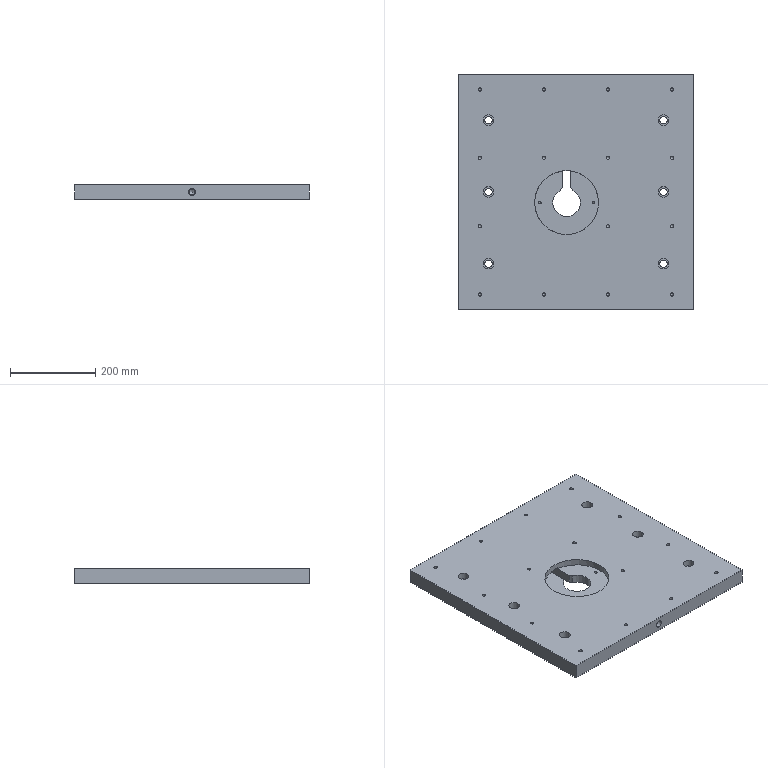Part | STEP file | 车灯-后视镜_id646_x_t | 1 solid | 108 faces | box 550 x 550 x 35 mm | volume 10040225 mm3 | cylinder 54 | plane 35 | cone 19 | commonest cylinder face diameters 6.9 x15 8 x15 17 x6 25 x6 5.1 x2 6 x2